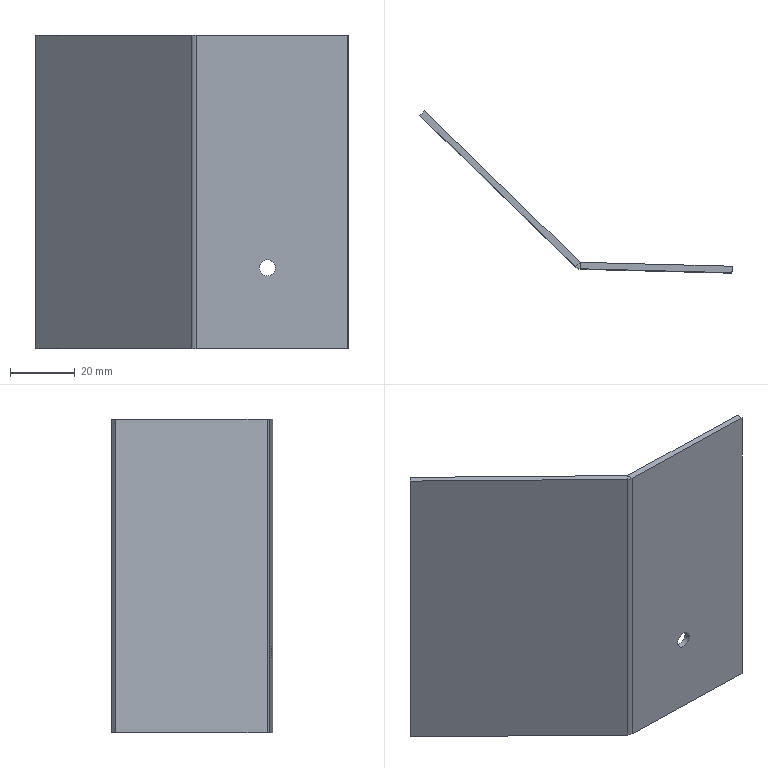Part | STEP file | Assembly TS-001-03 | 1 solid | 16 faces | box 96.717 x 50.15 x 97 mm | volume 22295 mm3 | plane 12 | cylinder 4 | commonest cylinder face diameters 5 x2 0.4 x1 4.4 x1
STEP:
#1=CARTESIAN_POINT('',(0.,0.,0.));
#2=DIRECTION('',(0.,0.,1.));
#3=DIRECTION('',(1.,0.,0.));
#4=AXIS2_PLACEMENT_3D('',#1,#2,#3);
#5=CARTESIAN_POINT('',(207.046,163.915,25.));
#6=VERTEX_POINT('',#5);
#7=CARTESIAN_POINT('',(207.098,165.914,25.));
#8=VERTEX_POINT('',#7);
#9=CARTESIAN_POINT('',(206.84,155.918,25.));
#10=DIRECTION('',(0.02576,0.9997,0.));
#11=VECTOR('',#10,1.);
#12=LINE('',#9,#11);
#13=CARTESIAN_POINT('',(209.34,155.853,25.));
#14=DIRECTION('',(0.02576,0.9997,0.));
#15=DIRECTION('',(-0.9997,0.02576,0.));
#16=AXIS2_PLACEMENT_3D('',#13,#14,#15);
#17=CYLINDRICAL_SURFACE('',#16,2.5);
#18=CARTESIAN_POINT('',(6.283,0.));
#19=DIRECTION('',(0.,1.));
#20=VECTOR('',#19,1.);
#21=LINE('',#18,#20);
#22=(GEOMETRIC_REPRESENTATION_CONTEXT(2)PARAMETRIC_REPRESENTATION_CONTEXT()REPRESENTATION_CONTEXT('',''));
#23=DEFINITIONAL_REPRESENTATION('',(#21),#22);
#24=PCURVE('',#17,#23);
#25=CARTESIAN_POINT('',(209.34,155.853,25.));
#26=DIRECTION('',(0.02576,0.9997,0.));
#27=DIRECTION('',(-0.9997,0.02576,0.));
#28=AXIS2_PLACEMENT_3D('',#25,#26,#27);
#29=CYLINDRICAL_SURFACE('',#28,2.5);
#30=CARTESIAN_POINT('',(0.,0.));
#31=DIRECTION('',(0.,1.));
#32=VECTOR('',#31,1.);
#33=LINE('',#30,#32);
#34=(GEOMETRIC_REPRESENTATION_CONTEXT(2)PARAMETRIC_REPRESENTATION_CONTEXT()REPRESENTATION_CONTEXT('',''));
#35=DEFINITIONAL_REPRESENTATION('',(#33),#34);
#36=PCURVE('',#29,#35);
#37=SURFACE_CURVE('',#12,(#24,#36),.PCURVE_S1.);
#38=EDGE_CURVE('',#6,#8,#37,.T.);
#39=ORIENTED_EDGE('',*,*,#38,.T.);
#40=CARTESIAN_POINT('',(212.096,165.785,25.));
#41=VERTEX_POINT('',#40);
#42=CARTESIAN_POINT('',(209.597,165.85,25.));
#43=DIRECTION('',(0.02576,0.9997,0.));
#44=DIRECTION('',(-0.9997,0.02576,0.));
#45=AXIS2_PLACEMENT_3D('',#42,#43,#44);
#46=CIRCLE('',#45,2.5);
#47=CARTESIAN_POINT('',(0.,10.));
#48=DIRECTION('',(1.,0.));
#49=VECTOR('',#48,1.);
#50=LINE('',#47,#49);
#51=(GEOMETRIC_REPRESENTATION_CONTEXT(2)PARAMETRIC_REPRESENTATION_CONTEXT()REPRESENTATION_CONTEXT('',''));
#52=DEFINITIONAL_REPRESENTATION('',(#50),#51);
#53=PCURVE('',#17,#52);
#54=CARTESIAN_POINT('',(234.589,165.206,97.));
#55=DIRECTION('',(-0.02576,-0.9997,0.));
#56=DIRECTION('',(0.9997,-0.02576,0.));
#57=AXIS2_PLACEMENT_3D('',#54,#55,#56);
#58=PLANE('',#57);
#59=CARTESIAN_POINT('',(-27.5,-72.));
#60=CARTESIAN_POINT('',(-27.5,-67.67));
#61=CARTESIAN_POINT('',(-23.75,-69.835));
#62=CARTESIAN_POINT('',(-20.,-72.));
#63=CARTESIAN_POINT('',(-23.75,-74.165));
#64=CARTESIAN_POINT('',(-27.5,-76.33));
#65=CARTESIAN_POINT('',(-27.5,-72.));
#66=(BOUNDED_CURVE()B_SPLINE_CURVE(2,(#59,#60,#61,#62,#63,#64,#65),.UNSPECIFIED.,.T.,.F.)B_SPLINE_CURVE_WITH_KNOTS((1,2,2,2,2,1),(-2.094,0.,2.094,4.189,6.283,8.378),.UNSPECIFIED.)CURVE()GEOMETRIC_REPRESENTATION_ITEM()RATIONAL_B_SPLINE_CURVE((1.,0.5,1.,0.5,1.,0.5,1.))REPRESENTATION_ITEM(''));
#67=(GEOMETRIC_REPRESENTATION_CONTEXT(2)PARAMETRIC_REPRESENTATION_CONTEXT()REPRESENTATION_CONTEXT('',''));
#68=DEFINITIONAL_REPRESENTATION('',(#66),#67);
#69=PCURVE('',#58,#68);
#70=SURFACE_CURVE('',#46,(#53,#69),.PCURVE_S1.);
#71=EDGE_CURVE('',#41,#8,#70,.T.);
#72=ORIENTED_EDGE('',*,*,#71,.F.);
#73=CARTESIAN_POINT('',(212.045,163.786,25.));
#74=VERTEX_POINT('',#73);
#75=CARTESIAN_POINT('',(211.839,155.789,25.));
#76=DIRECTION('',(0.02576,0.9997,0.));
#77=VECTOR('',#76,1.);
#78=LINE('',#75,#77);
#79=CARTESIAN_POINT('',(3.142,0.));
#80=DIRECTION('',(0.,1.));
#81=VECTOR('',#80,1.);
#82=LINE('',#79,#81);
#83=(GEOMETRIC_REPRESENTATION_CONTEXT(2)PARAMETRIC_REPRESENTATION_CONTEXT()REPRESENTATION_CONTEXT('',''));
#84=DEFINITIONAL_REPRESENTATION('',(#82),#83);
#85=PCURVE('',#17,#84);
#86=CARTESIAN_POINT('',(3.142,0.));
#87=DIRECTION('',(0.,1.));
#88=VECTOR('',#87,1.);
#89=LINE('',#86,#88);
#90=(GEOMETRIC_REPRESENTATION_CONTEXT(2)PARAMETRIC_REPRESENTATION_CONTEXT()REPRESENTATION_CONTEXT('',''));
#91=DEFINITIONAL_REPRESENTATION('',(#89),#90);
#92=PCURVE('',#29,#91);
#93=SURFACE_CURVE('',#78,(#85,#92),.PCURVE_S1.);
#94=EDGE_CURVE('',#74,#41,#93,.T.);
#95=ORIENTED_EDGE('',*,*,#94,.F.);
#96=CARTESIAN_POINT('',(209.546,163.85,25.));
#97=DIRECTION('',(-0.02576,-0.9997,0.));
#98=DIRECTION('',(0.9997,-0.02576,0.));
#99=AXIS2_PLACEMENT_3D('',#96,#97,#98);
#100=CIRCLE('',#99,2.5);
#101=CARTESIAN_POINT('',(9.425,8.));
#102=DIRECTION('',(-1.,0.));
#103=VECTOR('',#102,1.);
#104=LINE('',#101,#103);
#105=(GEOMETRIC_REPRESENTATION_CONTEXT(2)PARAMETRIC_REPRESENTATION_CONTEXT()REPRESENTATION_CONTEXT('',''));
#106=DEFINITIONAL_REPRESENTATION('',(#104),#105);
#107=PCURVE('',#17,#106);
#108=CARTESIAN_POINT('',(234.537,163.207,97.));
#109=DIRECTION('',(-0.02576,-0.9997,0.));
#110=DIRECTION('',(0.9997,-0.02576,0.));
#111=AXIS2_PLACEMENT_3D('',#108,#109,#110);
#112=PLANE('',#111);
#113=CARTESIAN_POINT('',(-25.,-72.));
#114=DIRECTION('',(1.,0.));
#115=AXIS2_PLACEMENT_2D('',#113,#114);
#116=CIRCLE('',#115,2.5);
#117=(GEOMETRIC_REPRESENTATION_CONTEXT(2)PARAMETRIC_REPRESENTATION_CONTEXT()REPRESENTATION_CONTEXT('',''));
#118=DEFINITIONAL_REPRESENTATION('',(#116),#117);
#119=PCURVE('',#112,#118);
#120=SURFACE_CURVE('',#100,(#107,#119),.PCURVE_S1.);
#121=EDGE_CURVE('',#6,#74,#120,.T.);
#122=ORIENTED_EDGE('',*,*,#121,.F.);
#123=EDGE_LOOP('',(#39,#72,#95,#122));
#124=FACE_BOUND('',#123,.F.);
#125=ADVANCED_FACE('',(#124),#17,.F.);
#126=CARTESIAN_POINT('',(186.126,165.037,97.));
#127=VERTEX_POINT('',#126);
#128=CARTESIAN_POINT('',(187.519,166.472,97.));
#129=VERTEX_POINT('',#128);
#130=CARTESIAN_POINT('',(186.126,165.037,97.));
#131=DIRECTION('',(0.6969,0.7172,0.));
#132=VECTOR('',#131,1.);
#133=LINE('',#130,#132);
#134=CARTESIAN_POINT('',(186.126,165.037,97.));
#135=DIRECTION('',(0.,0.,1.));
#136=DIRECTION('',(1.,0.,0.));
#137=AXIS2_PLACEMENT_3D('',#134,#135,#136);
#138=PLANE('',#137);
#139=CARTESIAN_POINT('',(0.,0.));
#140=DIRECTION('',(0.6969,0.7172));
#141=VECTOR('',#140,1.);
#142=LINE('',#139,#141);
#143=(GEOMETRIC_REPRESENTATION_CONTEXT(2)PARAMETRIC_REPRESENTATION_CONTEXT()REPRESENTATION_CONTEXT('',''));
#144=DEFINITIONAL_REPRESENTATION('',(#142),#143);
#145=PCURVE('',#138,#144);
#146=CARTESIAN_POINT('',(187.653,166.415,97.));
#147=DIRECTION('',(0.,0.,1.));
#148=DIRECTION('',(1.,0.,0.));
#149=AXIS2_PLACEMENT_3D('',#146,#147,#148);
#150=PLANE('',#149);
#151=CARTESIAN_POINT('',(-1.528,-1.378));
#152=DIRECTION('',(0.6969,0.7172));
#153=VECTOR('',#152,1.);
#154=LINE('',#151,#153);
#155=(GEOMETRIC_REPRESENTATION_CONTEXT(2)PARAMETRIC_REPRESENTATION_CONTEXT()REPRESENTATION_CONTEXT('',''));
#156=DEFINITIONAL_REPRESENTATION('',(#154),#155);
#157=PCURVE('',#150,#156);
#158=SURFACE_CURVE('',#133,(#145,#157),.PCURVE_S1.);
#159=EDGE_CURVE('',#127,#129,#158,.T.);
#160=ORIENTED_EDGE('',*,*,#159,.F.);
#161=CARTESIAN_POINT('',(187.602,164.416,97.));
#162=VERTEX_POINT('',#161);
#163=CARTESIAN_POINT('',(187.659,166.615,97.));
#164=DIRECTION('',(0.,0.,-1.));
#165=DIRECTION('',(1.,0.,0.));
#166=AXIS2_PLACEMENT_3D('',#163,#164,#165);
#167=CIRCLE('',#166,2.2);
#168=CARTESIAN_POINT('',(3.733,1.578));
#169=CARTESIAN_POINT('',(3.733,-2.233));
#170=CARTESIAN_POINT('',(0.4331,-0.3274));
#171=CARTESIAN_POINT('',(-2.867,1.578));
#172=CARTESIAN_POINT('',(0.4331,3.483));
#173=CARTESIAN_POINT('',(3.733,5.388));
#174=CARTESIAN_POINT('',(3.733,1.578));
#175=(BOUNDED_CURVE()B_SPLINE_CURVE(2,(#168,#169,#170,#171,#172,#173,#174),.UNSPECIFIED.,.T.,.F.)B_SPLINE_CURVE_WITH_KNOTS((1,2,2,2,2,1),(-2.094,0.,2.094,4.189,6.283,8.378),.UNSPECIFIED.)CURVE()GEOMETRIC_REPRESENTATION_ITEM()RATIONAL_B_SPLINE_CURVE((1.,0.5,1.,0.5,1.,0.5,1.))REPRESENTATION_ITEM(''));
#176=(GEOMETRIC_REPRESENTATION_CONTEXT(2)PARAMETRIC_REPRESENTATION_CONTEXT()REPRESENTATION_CONTEXT('',''));
#177=DEFINITIONAL_REPRESENTATION('',(#175),#176);
#178=PCURVE('',#138,#177);
#179=CARTESIAN_POINT('',(187.659,166.615,97.));
#180=DIRECTION('',(0.,0.,-1.));
#181=DIRECTION('',(-1.,0.,0.));
#182=AXIS2_PLACEMENT_3D('',#179,#180,#181);
#183=CYLINDRICAL_SURFACE('',#182,2.2);
#184=CARTESIAN_POINT('',(3.142,0.));
#185=DIRECTION('',(1.,0.));
#186=VECTOR('',#185,1.);
#187=LINE('',#184,#186);
#188=(GEOMETRIC_REPRESENTATION_CONTEXT(2)PARAMETRIC_REPRESENTATION_CONTEXT()REPRESENTATION_CONTEXT('',''));
#189=DEFINITIONAL_REPRESENTATION('',(#187),#188);
#190=PCURVE('',#183,#189);
#191=SURFACE_CURVE('',#167,(#178,#190),.PCURVE_S1.);
#192=EDGE_CURVE('',#162,#127,#191,.T.);
#193=ORIENTED_EDGE('',*,*,#192,.F.);
#194=CARTESIAN_POINT('',(187.653,166.415,97.));
#195=VERTEX_POINT('',#194);
#196=CARTESIAN_POINT('',(187.653,166.415,97.));
#197=DIRECTION('',(-0.02576,-0.9997,0.));
#198=VECTOR('',#197,1.);
#199=LINE('',#196,#198);
#200=CARTESIAN_POINT('',(1.528,1.378));
#201=DIRECTION('',(-0.02576,-0.9997));
#202=VECTOR('',#201,1.);
#203=LINE('',#200,#202);
#204=(GEOMETRIC_REPRESENTATION_CONTEXT(2)PARAMETRIC_REPRESENTATION_CONTEXT()REPRESENTATION_CONTEXT('',''));
#205=DEFINITIONAL_REPRESENTATION('',(#203),#204);
#206=PCURVE('',#138,#205);
#207=CARTESIAN_POINT('',(187.659,166.615,97.));
#208=DIRECTION('',(0.,0.,1.));
#209=DIRECTION('',(1.,0.,0.));
#210=AXIS2_PLACEMENT_3D('',#207,#208,#209);
#211=PLANE('',#210);
#212=CARTESIAN_POINT('',(-0.005151,-0.1999));
#213=DIRECTION('',(-0.02576,-0.9997));
#214=VECTOR('',#213,1.);
#215=LINE('',#212,#214);
#216=(GEOMETRIC_REPRESENTATION_CONTEXT(2)PARAMETRIC_REPRESENTATION_CONTEXT()REPRESENTATION_CONTEXT('',''));
#217=DEFINITIONAL_REPRESENTATION('',(#215),#216);
#218=PCURVE('',#211,#217);
#219=SURFACE_CURVE('',#199,(#206,#218),.PCURVE_S1.);
#220=EDGE_CURVE('',#195,#162,#219,.T.);
#221=ORIENTED_EDGE('',*,*,#220,.F.);
#222=CARTESIAN_POINT('',(187.659,166.615,97.));
#223=DIRECTION('',(0.,0.,-1.));
#224=DIRECTION('',(1.,0.,0.));
#225=AXIS2_PLACEMENT_3D('',#222,#223,#224);
#226=CIRCLE('',#225,0.2);
#227=CARTESIAN_POINT('',(1.733,1.578));
#228=CARTESIAN_POINT('',(1.733,1.231));
#229=CARTESIAN_POINT('',(1.433,1.405));
#230=CARTESIAN_POINT('',(1.133,1.578));
#231=CARTESIAN_POINT('',(1.433,1.751));
#232=CARTESIAN_POINT('',(1.733,1.924));
#233=CARTESIAN_POINT('',(1.733,1.578));
#234=(BOUNDED_CURVE()B_SPLINE_CURVE(2,(#227,#228,#229,#230,#231,#232,#233),.UNSPECIFIED.,.T.,.F.)B_SPLINE_CURVE_WITH_KNOTS((1,2,2,2,2,1),(-2.094,0.,2.094,4.189,6.283,8.378),.UNSPECIFIED.)CURVE()GEOMETRIC_REPRESENTATION_ITEM()RATIONAL_B_SPLINE_CURVE((1.,0.5,1.,0.5,1.,0.5,1.))REPRESENTATION_ITEM(''));
#235=(GEOMETRIC_REPRESENTATION_CONTEXT(2)PARAMETRIC_REPRESENTATION_CONTEXT()REPRESENTATION_CONTEXT('',''));
#236=DEFINITIONAL_REPRESENTATION('',(#234),#235);
#237=PCURVE('',#138,#236);
#238=CARTESIAN_POINT('',(187.659,166.615,97.));
#239=DIRECTION('',(0.,0.,-1.));
#240=DIRECTION('',(-1.,0.,0.));
#241=AXIS2_PLACEMENT_3D('',#238,#239,#240);
#242=CYLINDRICAL_SURFACE('',#241,0.2);
#243=CARTESIAN_POINT('',(3.142,0.));
#244=DIRECTION('',(1.,0.));
#245=VECTOR('',#244,1.);
#246=LINE('',#243,#245);
#247=(GEOMETRIC_REPRESENTATION_CONTEXT(2)PARAMETRIC_REPRESENTATION_CONTEXT()REPRESENTATION_CONTEXT('',''));
#248=DEFINITIONAL_REPRESENTATION('',(#246),#247);
#249=PCURVE('',#242,#248);
#250=SURFACE_CURVE('',#226,(#237,#249),.PCURVE_S1.);
#251=EDGE_CURVE('',#195,#129,#250,.T.);
#252=ORIENTED_EDGE('',*,*,#251,.T.);
#253=EDGE_LOOP('',(#160,#193,#221,#252));
#254=FACE_BOUND('',#253,.T.);
#255=ADVANCED_FACE('',(#254),#138,.T.);
#256=CARTESIAN_POINT('',(137.872,211.922,97.));
#257=VERTEX_POINT('',#256);
#258=CARTESIAN_POINT('',(186.742,164.438,97.));
#259=DIRECTION('',(-0.7172,0.6969,0.));
#260=VECTOR('',#259,1.);
#261=LINE('',#258,#260);
#262=CARTESIAN_POINT('',(-0.9112,-1.977));
#263=DIRECTION('',(-0.7172,0.6969));
#264=VECTOR('',#263,1.);
#265=LINE('',#262,#264);
#266=(GEOMETRIC_REPRESENTATION_CONTEXT(2)PARAMETRIC_REPRESENTATION_CONTEXT()REPRESENTATION_CONTEXT('',''));
#267=DEFINITIONAL_REPRESENTATION('',(#265),#266);
#268=PCURVE('',#150,#267);
#269=CARTESIAN_POINT('',(186.742,164.438,97.));
#270=DIRECTION('',(-0.6969,-0.7172,0.));
#271=DIRECTION('',(0.7172,-0.6969,0.));
#272=AXIS2_PLACEMENT_3D('',#269,#270,#271);
#273=PLANE('',#272);
#274=CARTESIAN_POINT('',(0.,0.));
#275=DIRECTION('',(-1.,0.));
#276=VECTOR('',#275,1.);
#277=LINE('',#274,#276);
#278=(GEOMETRIC_REPRESENTATION_CONTEXT(2)PARAMETRIC_REPRESENTATION_CONTEXT()REPRESENTATION_CONTEXT('',''));
#279=DEFINITIONAL_REPRESENTATION('',(#277),#278);
#280=PCURVE('',#273,#279);
#281=SURFACE_CURVE('',#261,(#268,#280),.PCURVE_S1.);
#282=EDGE_CURVE('',#127,#257,#281,.T.);
#283=ORIENTED_EDGE('',*,*,#282,.F.);
#284=ORIENTED_EDGE('',*,*,#159,.T.);
#285=CARTESIAN_POINT('',(139.266,213.357,97.));
#286=VERTEX_POINT('',#285);
#287=CARTESIAN_POINT('',(188.136,165.872,97.));
#288=DIRECTION('',(-0.7172,0.6969,0.));
#289=VECTOR('',#288,1.);
#290=LINE('',#287,#289);
#291=CARTESIAN_POINT('',(0.4825,-0.5428));
#292=DIRECTION('',(-0.7172,0.6969));
#293=VECTOR('',#292,1.);
#294=LINE('',#291,#293);
#295=(GEOMETRIC_REPRESENTATION_CONTEXT(2)PARAMETRIC_REPRESENTATION_CONTEXT()REPRESENTATION_CONTEXT('',''));
#296=DEFINITIONAL_REPRESENTATION('',(#294),#295);
#297=PCURVE('',#150,#296);
#298=CARTESIAN_POINT('',(188.136,165.872,97.));
#299=DIRECTION('',(-0.6969,-0.7172,0.));
#300=DIRECTION('',(0.7172,-0.6969,0.));
#301=AXIS2_PLACEMENT_3D('',#298,#299,#300);
#302=PLANE('',#301);
#303=CARTESIAN_POINT('',(0.,0.));
#304=DIRECTION('',(-1.,0.));
#305=VECTOR('',#304,1.);
#306=LINE('',#303,#305);
#307=(GEOMETRIC_REPRESENTATION_CONTEXT(2)PARAMETRIC_REPRESENTATION_CONTEXT()REPRESENTATION_CONTEXT('',''));
#308=DEFINITIONAL_REPRESENTATION('',(#306),#307);
#309=PCURVE('',#302,#308);
#310=SURFACE_CURVE('',#290,(#297,#309),.PCURVE_S1.);
#311=EDGE_CURVE('',#129,#286,#310,.T.);
#312=ORIENTED_EDGE('',*,*,#311,.T.);
#313=CARTESIAN_POINT('',(137.872,211.922,97.));
#314=DIRECTION('',(0.6969,0.7172,0.));
#315=VECTOR('',#314,1.);
#316=LINE('',#313,#315);
#317=CARTESIAN_POINT('',(-49.781,45.507));
#318=DIRECTION('',(0.6969,0.7172));
#319=VECTOR('',#318,1.);
#320=LINE('',#317,#319);
#321=(GEOMETRIC_REPRESENTATION_CONTEXT(2)PARAMETRIC_REPRESENTATION_CONTEXT()REPRESENTATION_CONTEXT('',''));
#322=DEFINITIONAL_REPRESENTATION('',(#320),#321);
#323=PCURVE('',#150,#322);
#324=CARTESIAN_POINT('',(137.872,211.922,97.));
#325=DIRECTION('',(-0.7172,0.6969,0.));
#326=DIRECTION('',(-0.6969,-0.7172,0.));
#327=AXIS2_PLACEMENT_3D('',#324,#325,#326);
#328=PLANE('',#327);
#329=CARTESIAN_POINT('',(0.,0.));
#330=DIRECTION('',(-1.,0.));
#331=VECTOR('',#330,1.);
#332=LINE('',#329,#331);
#333=(GEOMETRIC_REPRESENTATION_CONTEXT(2)PARAMETRIC_REPRESENTATION_CONTEXT()REPRESENTATION_CONTEXT('',''));
#334=DEFINITIONAL_REPRESENTATION('',(#332),#333);
#335=PCURVE('',#328,#334);
#336=SURFACE_CURVE('',#316,(#323,#335),.PCURVE_S1.);
#337=EDGE_CURVE('',#257,#286,#336,.T.);
#338=ORIENTED_EDGE('',*,*,#337,.F.);
#339=EDGE_LOOP('',(#283,#284,#312,#338));
#340=FACE_BOUND('',#339,.T.);
#341=ADVANCED_FACE('',(#340),#150,.T.);
#342=CARTESIAN_POINT('',(187.602,164.416,0.));
#343=VERTEX_POINT('',#342);
#344=CARTESIAN_POINT('',(187.653,166.415,0.));
#345=VERTEX_POINT('',#344);
#346=CARTESIAN_POINT('',(187.602,164.416,0.));
#347=DIRECTION('',(0.02576,0.9997,0.));
#348=VECTOR('',#347,1.);
#349=LINE('',#346,#348);
#350=CARTESIAN_POINT('',(187.602,164.416,0.));
#351=DIRECTION('',(0.,0.,-1.));
#352=DIRECTION('',(-1.,0.,0.));
#353=AXIS2_PLACEMENT_3D('',#350,#351,#352);
#354=PLANE('',#353);
#355=CARTESIAN_POINT('',(0.,0.));
#356=DIRECTION('',(-0.02576,0.9997));
#357=VECTOR('',#356,1.);
#358=LINE('',#355,#357);
#359=(GEOMETRIC_REPRESENTATION_CONTEXT(2)PARAMETRIC_REPRESENTATION_CONTEXT()REPRESENTATION_CONTEXT('',''));
#360=DEFINITIONAL_REPRESENTATION('',(#358),#359);
#361=PCURVE('',#354,#360);
#362=CARTESIAN_POINT('',(187.519,166.472,0.));
#363=DIRECTION('',(0.,0.,-1.));
#364=DIRECTION('',(-1.,0.,0.));
#365=AXIS2_PLACEMENT_3D('',#362,#363,#364);
#366=PLANE('',#365);
#367=CARTESIAN_POINT('',(-0.08271,-2.056));
#368=DIRECTION('',(-0.02576,0.9997));
#369=VECTOR('',#368,1.);
#370=LINE('',#367,#369);
#371=(GEOMETRIC_REPRESENTATION_CONTEXT(2)PARAMETRIC_REPRESENTATION_CONTEXT()REPRESENTATION_CONTEXT('',''));
#372=DEFINITIONAL_REPRESENTATION('',(#370),#371);
#373=PCURVE('',#366,#372);
#374=SURFACE_CURVE('',#349,(#361,#373),.PCURVE_S1.);
#375=EDGE_CURVE('',#343,#345,#374,.T.);
#376=ORIENTED_EDGE('',*,*,#375,.F.);
#377=CARTESIAN_POINT('',(186.126,165.037,0.));
#378=VERTEX_POINT('',#377);
#379=CARTESIAN_POINT('',(187.659,166.615,0.));
#380=DIRECTION('',(0.,0.,-1.));
#381=DIRECTION('',(1.,0.,0.));
#382=AXIS2_PLACEMENT_3D('',#379,#380,#381);
#383=CIRCLE('',#382,2.2);
#384=CARTESIAN_POINT('',(-0.05666,2.199));
#385=DIRECTION('',(-1.,0.));
#386=AXIS2_PLACEMENT_2D('',#384,#385);
#387=CIRCLE('',#386,2.2);
#388=(GEOMETRIC_REPRESENTATION_CONTEXT(2)PARAMETRIC_REPRESENTATION_CONTEXT()REPRESENTATION_CONTEXT('',''));
#389=DEFINITIONAL_REPRESENTATION('',(#387),#388);
#390=PCURVE('',#354,#389);
#391=CARTESIAN_POINT('',(3.142,97.));
#392=DIRECTION('',(1.,0.));
#393=VECTOR('',#392,1.);
#394=LINE('',#391,#393);
#395=(GEOMETRIC_REPRESENTATION_CONTEXT(2)PARAMETRIC_REPRESENTATION_CONTEXT()REPRESENTATION_CONTEXT('',''));
#396=DEFINITIONAL_REPRESENTATION('',(#394),#395);
#397=PCURVE('',#183,#396);
#398=SURFACE_CURVE('',#383,(#390,#397),.PCURVE_S1.);
#399=EDGE_CURVE('',#343,#378,#398,.T.);
#400=ORIENTED_EDGE('',*,*,#399,.T.);
#401=CARTESIAN_POINT('',(187.519,166.472,0.));
#402=VERTEX_POINT('',#401);
#403=CARTESIAN_POINT('',(187.519,166.472,0.));
#404=DIRECTION('',(-0.6969,-0.7172,0.));
#405=VECTOR('',#404,1.);
#406=LINE('',#403,#405);
#407=CARTESIAN_POINT('',(0.08271,2.056));
#408=DIRECTION('',(0.6969,-0.7172));
#409=VECTOR('',#408,1.);
#410=LINE('',#407,#409);
#411=(GEOMETRIC_REPRESENTATION_CONTEXT(2)PARAMETRIC_REPRESENTATION_CONTEXT()REPRESENTATION_CONTEXT('',''));
#412=DEFINITIONAL_REPRESENTATION('',(#410),#411);
#413=PCURVE('',#354,#412);
#414=CARTESIAN_POINT('',(187.659,166.615,0.));
#415=DIRECTION('',(0.,0.,1.));
#416=DIRECTION('',(1.,0.,0.));
#417=AXIS2_PLACEMENT_3D('',#414,#415,#416);
#418=PLANE('',#417);
#419=CARTESIAN_POINT('',(-0.1394,-0.1434));
#420=DIRECTION('',(-0.6969,-0.7172));
#421=VECTOR('',#420,1.);
#422=LINE('',#419,#421);
#423=(GEOMETRIC_REPRESENTATION_CONTEXT(2)PARAMETRIC_REPRESENTATION_CONTEXT()REPRESENTATION_CONTEXT('',''));
#424=DEFINITIONAL_REPRESENTATION('',(#422),#423);
#425=PCURVE('',#418,#424);
#426=SURFACE_CURVE('',#406,(#413,#425),.PCURVE_S1.);
#427=EDGE_CURVE('',#402,#378,#426,.T.);
#428=ORIENTED_EDGE('',*,*,#427,.F.);
#429=CARTESIAN_POINT('',(187.659,166.615,0.));
#430=DIRECTION('',(0.,0.,-1.));
#431=DIRECTION('',(1.,0.,0.));
#432=AXIS2_PLACEMENT_3D('',#429,#430,#431);
#433=CIRCLE('',#432,0.2);
#434=CARTESIAN_POINT('',(-0.05666,2.199));
#435=DIRECTION('',(-1.,0.));
#436=AXIS2_PLACEMENT_2D('',#434,#435);
#437=CIRCLE('',#436,0.2);
#438=(GEOMETRIC_REPRESENTATION_CONTEXT(2)PARAMETRIC_REPRESENTATION_CONTEXT()REPRESENTATION_CONTEXT('',''));
#439=DEFINITIONAL_REPRESENTATION('',(#437),#438);
#440=PCURVE('',#354,#439);
#441=CARTESIAN_POINT('',(3.142,97.));
#442=DIRECTION('',(1.,0.));
#443=VECTOR('',#442,1.);
#444=LINE('',#441,#443);
#445=(GEOMETRIC_REPRESENTATION_CONTEXT(2)PARAMETRIC_REPRESENTATION_CONTEXT()REPRESENTATION_CONTEXT('',''));
#446=DEFINITIONAL_REPRESENTATION('',(#444),#445);
#447=PCURVE('',#242,#446);
#448=SURFACE_CURVE('',#433,(#440,#447),.PCURVE_S1.);
#449=EDGE_CURVE('',#345,#402,#448,.T.);
#450=ORIENTED_EDGE('',*,*,#449,.F.);
#451=EDGE_LOOP('',(#376,#400,#428,#450));
#452=FACE_BOUND('',#451,.T.);
#453=ADVANCED_FACE('',(#452),#354,.T.);
#454=CARTESIAN_POINT('',(234.537,163.207,0.));
#455=VERTEX_POINT('',#454);
#456=CARTESIAN_POINT('',(234.537,163.207,0.));
#457=DIRECTION('',(-0.9997,0.02576,0.));
#458=VECTOR('',#457,1.);
#459=LINE('',#456,#458);
#460=CARTESIAN_POINT('',(-47.018,-3.265));
#461=DIRECTION('',(0.9997,0.02576));
#462=VECTOR('',#461,1.);
#463=LINE('',#460,#462);
#464=(GEOMETRIC_REPRESENTATION_CONTEXT(2)PARAMETRIC_REPRESENTATION_CONTEXT()REPRESENTATION_CONTEXT('',''));
#465=DEFINITIONAL_REPRESENTATION('',(#463),#464);
#466=PCURVE('',#366,#465);
#467=CARTESIAN_POINT('',(0.,-97.));
#468=DIRECTION('',(-1.,0.));
#469=VECTOR('',#468,1.);
#470=LINE('',#467,#469);
#471=(GEOMETRIC_REPRESENTATION_CONTEXT(2)PARAMETRIC_REPRESENTATION_CONTEXT()REPRESENTATION_CONTEXT('',''));
#472=DEFINITIONAL_REPRESENTATION('',(#470),#471);
#473=PCURVE('',#112,#472);
#474=SURFACE_CURVE('',#459,(#466,#473),.PCURVE_S1.);
#475=EDGE_CURVE('',#455,#343,#474,.T.);
#476=ORIENTED_EDGE('',*,*,#475,.T.);
#477=ORIENTED_EDGE('',*,*,#375,.T.);
#478=CARTESIAN_POINT('',(234.589,165.206,0.));
#479=VERTEX_POINT('',#478);
#480=CARTESIAN_POINT('',(234.589,165.206,0.));
#481=DIRECTION('',(-0.9997,0.02576,0.));
#482=VECTOR('',#481,1.);
#483=LINE('',#480,#482);
#484=CARTESIAN_POINT('',(-47.07,-1.266));
#485=DIRECTION('',(0.9997,0.02576));
#486=VECTOR('',#485,1.);
#487=LINE('',#484,#486);
#488=(GEOMETRIC_REPRESENTATION_CONTEXT(2)PARAMETRIC_REPRESENTATION_CONTEXT()REPRESENTATION_CONTEXT('',''));
#489=DEFINITIONAL_REPRESENTATION('',(#487),#488);
#490=PCURVE('',#366,#489);
#491=CARTESIAN_POINT('',(0.,-97.));
#492=DIRECTION('',(-1.,0.));
#493=VECTOR('',#492,1.);
#494=LINE('',#491,#493);
#495=(GEOMETRIC_REPRESENTATION_CONTEXT(2)PARAMETRIC_REPRESENTATION_CONTEXT()REPRESENTATION_CONTEXT('',''));
#496=DEFINITIONAL_REPRESENTATION('',(#494),#495);
#497=PCURVE('',#58,#496);
#498=SURFACE_CURVE('',#483,(#490,#497),.PCURVE_S1.);
#499=EDGE_CURVE('',#479,#345,#498,.T.);
#500=ORIENTED_EDGE('',*,*,#499,.F.);
#501=CARTESIAN_POINT('',(234.589,165.206,0.));
#502=DIRECTION('',(-0.02576,-0.9997,0.));
#503=VECTOR('',#502,1.);
#504=LINE('',#501,#503);
#505=CARTESIAN_POINT('',(-47.07,-1.266));
#506=DIRECTION('',(0.02576,-0.9997));
#507=VECTOR('',#506,1.);
#508=LINE('',#505,#507);
#509=(GEOMETRIC_REPRESENTATION_CONTEXT(2)PARAMETRIC_REPRESENTATION_CONTEXT()REPRESENTATION_CONTEXT('',''));
#510=DEFINITIONAL_REPRESENTATION('',(#508),#509);
#511=PCURVE('',#366,#510);
#512=CARTESIAN_POINT('',(234.589,165.206,97.));
#513=DIRECTION('',(0.9997,-0.02576,0.));
#514=DIRECTION('',(0.02576,0.9997,0.));
#515=AXIS2_PLACEMENT_3D('',#512,#513,#514);
#516=PLANE('',#515);
#517=CARTESIAN_POINT('',(0.,-97.));
#518=DIRECTION('',(-1.,0.));
#519=VECTOR('',#518,1.);
#520=LINE('',#517,#519);
#521=(GEOMETRIC_REPRESENTATION_CONTEXT(2)PARAMETRIC_REPRESENTATION_CONTEXT()REPRESENTATION_CONTEXT('',''));
#522=DEFINITIONAL_REPRESENTATION('',(#520),#521);
#523=PCURVE('',#516,#522);
#524=SURFACE_CURVE('',#504,(#511,#523),.PCURVE_S1.);
#525=EDGE_CURVE('',#479,#455,#524,.T.);
#526=ORIENTED_EDGE('',*,*,#525,.T.);
#527=EDGE_LOOP('',(#476,#477,#500,#526));
#528=FACE_BOUND('',#527,.T.);
#529=ADVANCED_FACE('',(#528),#366,.T.);
#530=CARTESIAN_POINT('',(139.266,213.357,0.));
#531=VERTEX_POINT('',#530);
#532=CARTESIAN_POINT('',(188.136,165.872,0.));
#533=DIRECTION('',(-0.7172,0.6969,0.));
#534=VECTOR('',#533,1.);
#535=LINE('',#532,#534);
#536=CARTESIAN_POINT('',(0.,-97.));
#537=DIRECTION('',(-1.,0.));
#538=VECTOR('',#537,1.);
#539=LINE('',#536,#538);
#540=(GEOMETRIC_REPRESENTATION_CONTEXT(2)PARAMETRIC_REPRESENTATION_CONTEXT()REPRESENTATION_CONTEXT('',''));
#541=DEFINITIONAL_REPRESENTATION('',(#539),#540);
#542=PCURVE('',#302,#541);
#543=CARTESIAN_POINT('',(0.4774,-0.7427));
#544=DIRECTION('',(-0.7172,0.6969));
#545=VECTOR('',#544,1.);
#546=LINE('',#543,#545);
#547=(GEOMETRIC_REPRESENTATION_CONTEXT(2)PARAMETRIC_REPRESENTATION_CONTEXT()REPRESENTATION_CONTEXT('',''));
#548=DEFINITIONAL_REPRESENTATION('',(#546),#547);
#549=PCURVE('',#418,#548);
#550=SURFACE_CURVE('',#535,(#542,#549),.PCURVE_S1.);
#551=EDGE_CURVE('',#402,#531,#550,.T.);
#552=ORIENTED_EDGE('',*,*,#551,.T.);
#553=CARTESIAN_POINT('',(139.266,213.357,97.));
#554=DIRECTION('',(0.,0.,-1.));
#555=VECTOR('',#554,1.);
#556=LINE('',#553,#555);
#557=CARTESIAN_POINT('',(-68.14,0.));
#558=DIRECTION('',(0.,-1.));
#559=VECTOR('',#558,1.);
#560=LINE('',#557,#559);
#561=(GEOMETRIC_REPRESENTATION_CONTEXT(2)PARAMETRIC_REPRESENTATION_CONTEXT()REPRESENTATION_CONTEXT('',''));
#562=DEFINITIONAL_REPRESENTATION('',(#560),#561);
#563=PCURVE('',#302,#562);
#564=CARTESIAN_POINT('',(-2.,0.));
#565=DIRECTION('',(0.,-1.));
#566=VECTOR('',#565,1.);
#567=LINE('',#564,#566);
#568=(GEOMETRIC_REPRESENTATION_CONTEXT(2)PARAMETRIC_REPRESENTATION_CONTEXT()REPRESENTATION_CONTEXT('',''));
#569=DEFINITIONAL_REPRESENTATION('',(#567),#568);
#570=PCURVE('',#328,#569);
#571=SURFACE_CURVE('',#556,(#563,#570),.PCURVE_S1.);
#572=EDGE_CURVE('',#286,#531,#571,.T.);
#573=ORIENTED_EDGE('',*,*,#572,.F.);
#574=ORIENTED_EDGE('',*,*,#311,.F.);
#575=CARTESIAN_POINT('',(187.519,166.472,97.));
#576=DIRECTION('',(0.,0.,-1.));
#577=VECTOR('',#576,1.);
#578=LINE('',#575,#577);
#579=CARTESIAN_POINT('',(-0.86,0.));
#580=DIRECTION('',(0.,-1.));
#581=VECTOR('',#580,1.);
#582=LINE('',#579,#581);
#583=(GEOMETRIC_REPRESENTATION_CONTEXT(2)PARAMETRIC_REPRESENTATION_CONTEXT()REPRESENTATION_CONTEXT('',''));
#584=DEFINITIONAL_REPRESENTATION('',(#582),#583);
#585=PCURVE('',#302,#584);
#586=CARTESIAN_POINT('',(5.483,0.));
#587=DIRECTION('',(0.,1.));
#588=VECTOR('',#587,1.);
#589=LINE('',#586,#588);
#590=(GEOMETRIC_REPRESENTATION_CONTEXT(2)PARAMETRIC_REPRESENTATION_CONTEXT()REPRESENTATION_CONTEXT('',''));
#591=DEFINITIONAL_REPRESENTATION('',(#589),#590);
#592=PCURVE('',#242,#591);
#593=SURFACE_CURVE('',#578,(#585,#592),.PCURVE_S1.);
#594=EDGE_CURVE('',#129,#402,#593,.T.);
#595=ORIENTED_EDGE('',*,*,#594,.T.);
#596=EDGE_LOOP('',(#552,#573,#574,#595));
#597=FACE_BOUND('',#596,.T.);
#598=ADVANCED_FACE('',(#597),#302,.F.);
#599=CARTESIAN_POINT('',(137.872,211.922,0.));
#600=VERTEX_POINT('',#599);
#601=CARTESIAN_POINT('',(137.872,211.922,0.));
#602=DIRECTION('',(0.6969,0.7172,0.));
#603=VECTOR('',#602,1.);
#604=LINE('',#601,#603);
#605=CARTESIAN_POINT('',(0.,-97.));
#606=DIRECTION('',(-1.,0.));
#607=VECTOR('',#606,1.);
#608=LINE('',#605,#607);
#609=(GEOMETRIC_REPRESENTATION_CONTEXT(2)PARAMETRIC_REPRESENTATION_CONTEXT()REPRESENTATION_CONTEXT('',''));
#610=DEFINITIONAL_REPRESENTATION('',(#608),#609);
#611=PCURVE('',#328,#610);
#612=CARTESIAN_POINT('',(-49.787,45.307));
#613=DIRECTION('',(0.6969,0.7172));
#614=VECTOR('',#613,1.);
#615=LINE('',#612,#614);
#616=(GEOMETRIC_REPRESENTATION_CONTEXT(2)PARAMETRIC_REPRESENTATION_CONTEXT()REPRESENTATION_CONTEXT('',''));
#617=DEFINITIONAL_REPRESENTATION('',(#615),#616);
#618=PCURVE('',#418,#617);
#619=SURFACE_CURVE('',#604,(#611,#618),.PCURVE_S1.);
#620=EDGE_CURVE('',#600,#531,#619,.T.);
#621=ORIENTED_EDGE('',*,*,#620,.F.);
#622=CARTESIAN_POINT('',(137.872,211.922,97.));
#623=DIRECTION('',(0.,0.,-1.));
#624=VECTOR('',#623,1.);
#625=LINE('',#622,#624);
#626=CARTESIAN_POINT('',(0.,0.));
#627=DIRECTION('',(0.,-1.));
#628=VECTOR('',#627,1.);
#629=LINE('',#626,#628);
#630=(GEOMETRIC_REPRESENTATION_CONTEXT(2)PARAMETRIC_REPRESENTATION_CONTEXT()REPRESENTATION_CONTEXT('',''));
#631=DEFINITIONAL_REPRESENTATION('',(#629),#630);
#632=PCURVE('',#328,#631);
#633=CARTESIAN_POINT('',(-68.14,0.));
#634=DIRECTION('',(0.,-1.));
#635=VECTOR('',#634,1.);
#636=LINE('',#633,#635);
#637=(GEOMETRIC_REPRESENTATION_CONTEXT(2)PARAMETRIC_REPRESENTATION_CONTEXT()REPRESENTATION_CONTEXT('',''));
#638=DEFINITIONAL_REPRESENTATION('',(#636),#637);
#639=PCURVE('',#273,#638);
#640=SURFACE_CURVE('',#625,(#632,#639),.PCURVE_S1.);
#641=EDGE_CURVE('',#257,#600,#640,.T.);
#642=ORIENTED_EDGE('',*,*,#641,.F.);
#643=ORIENTED_EDGE('',*,*,#337,.T.);
#644=ORIENTED_EDGE('',*,*,#572,.T.);
#645=EDGE_LOOP('',(#621,#642,#643,#644));
#646=FACE_BOUND('',#645,.T.);
#647=ADVANCED_FACE('',(#646),#328,.T.);
#648=CARTESIAN_POINT('',(186.742,164.438,0.));
#649=DIRECTION('',(-0.7172,0.6969,0.));
#650=VECTOR('',#649,1.);
#651=LINE('',#648,#650);
#652=CARTESIAN_POINT('',(0.,-97.));
#653=DIRECTION('',(-1.,0.));
#654=VECTOR('',#653,1.);
#655=LINE('',#652,#654);
#656=(GEOMETRIC_REPRESENTATION_CONTEXT(2)PARAMETRIC_REPRESENTATION_CONTEXT()REPRESENTATION_CONTEXT('',''));
#657=DEFINITIONAL_REPRESENTATION('',(#655),#656);
#658=PCURVE('',#273,#657);
#659=CARTESIAN_POINT('',(-0.9163,-2.177));
#660=DIRECTION('',(-0.7172,0.6969));
#661=VECTOR('',#660,1.);
#662=LINE('',#659,#661);
#663=(GEOMETRIC_REPRESENTATION_CONTEXT(2)PARAMETRIC_REPRESENTATION_CONTEXT()REPRESENTATION_CONTEXT('',''));
#664=DEFINITIONAL_REPRESENTATION('',(#662),#663);
#665=PCURVE('',#418,#664);
#666=SURFACE_CURVE('',#651,(#658,#665),.PCURVE_S1.);
#667=EDGE_CURVE('',#378,#600,#666,.T.);
#668=ORIENTED_EDGE('',*,*,#667,.F.);
#669=CARTESIAN_POINT('',(186.126,165.037,97.));
#670=DIRECTION('',(0.,0.,-1.));
#671=VECTOR('',#670,1.);
#672=LINE('',#669,#671);
#673=CARTESIAN_POINT('',(-0.86,0.));
#674=DIRECTION('',(0.,-1.));
#675=VECTOR('',#674,1.);
#676=LINE('',#673,#675);
#677=(GEOMETRIC_REPRESENTATION_CONTEXT(2)PARAMETRIC_REPRESENTATION_CONTEXT()REPRESENTATION_CONTEXT('',''));
#678=DEFINITIONAL_REPRESENTATION('',(#676),#677);
#679=PCURVE('',#273,#678);
#680=CARTESIAN_POINT('',(5.483,0.));
#681=DIRECTION('',(0.,1.));
#682=VECTOR('',#681,1.);
#683=LINE('',#680,#682);
#684=(GEOMETRIC_REPRESENTATION_CONTEXT(2)PARAMETRIC_REPRESENTATION_CONTEXT()REPRESENTATION_CONTEXT('',''));
#685=DEFINITIONAL_REPRESENTATION('',(#683),#684);
#686=PCURVE('',#183,#685);
#687=SURFACE_CURVE('',#672,(#679,#686),.PCURVE_S1.);
#688=EDGE_CURVE('',#127,#378,#687,.T.);
#689=ORIENTED_EDGE('',*,*,#688,.F.);
#690=ORIENTED_EDGE('',*,*,#282,.T.);
#691=ORIENTED_EDGE('',*,*,#641,.T.);
#692=EDGE_LOOP('',(#668,#689,#690,#691));
#693=FACE_BOUND('',#692,.T.);
#694=ADVANCED_FACE('',(#693),#273,.T.);
#695=ORIENTED_EDGE('',*,*,#399,.F.);
#696=CARTESIAN_POINT('',(187.602,164.416,97.));
#697=DIRECTION('',(0.,0.,-1.));
#698=VECTOR('',#697,1.);
#699=LINE('',#696,#698);
#700=CARTESIAN_POINT('',(4.738,0.));
#701=DIRECTION('',(0.,1.));
#702=VECTOR('',#701,1.);
#703=LINE('',#700,#702);
#704=(GEOMETRIC_REPRESENTATION_CONTEXT(2)PARAMETRIC_REPRESENTATION_CONTEXT()REPRESENTATION_CONTEXT('',''));
#705=DEFINITIONAL_REPRESENTATION('',(#703),#704);
#706=PCURVE('',#183,#705);
#707=CARTESIAN_POINT('',(-46.951,0.));
#708=DIRECTION('',(0.,-1.));
#709=VECTOR('',#708,1.);
#710=LINE('',#707,#709);
#711=(GEOMETRIC_REPRESENTATION_CONTEXT(2)PARAMETRIC_REPRESENTATION_CONTEXT()REPRESENTATION_CONTEXT('',''));
#712=DEFINITIONAL_REPRESENTATION('',(#710),#711);
#713=PCURVE('',#112,#712);
#714=SURFACE_CURVE('',#699,(#706,#713),.PCURVE_S1.);
#715=EDGE_CURVE('',#162,#343,#714,.T.);
#716=ORIENTED_EDGE('',*,*,#715,.F.);
#717=ORIENTED_EDGE('',*,*,#192,.T.);
#718=ORIENTED_EDGE('',*,*,#688,.T.);
#719=EDGE_LOOP('',(#695,#716,#717,#718));
#720=FACE_BOUND('',#719,.T.);
#721=ADVANCED_FACE('',(#720),#183,.T.);
#722=ORIENTED_EDGE('',*,*,#121,.F.);
#723=CARTESIAN_POINT('',(209.546,163.85,25.));
#724=DIRECTION('',(-0.02576,-0.9997,0.));
#725=DIRECTION('',(0.9997,-0.02576,0.));
#726=AXIS2_PLACEMENT_3D('',#723,#724,#725);
#727=CIRCLE('',#726,2.5);
#728=CARTESIAN_POINT('',(-25.,-72.));
#729=DIRECTION('',(1.,0.));
#730=AXIS2_PLACEMENT_2D('',#728,#729);
#731=CIRCLE('',#730,2.5);
#732=(GEOMETRIC_REPRESENTATION_CONTEXT(2)PARAMETRIC_REPRESENTATION_CONTEXT()REPRESENTATION_CONTEXT('',''));
#733=DEFINITIONAL_REPRESENTATION('',(#731),#732);
#734=PCURVE('',#112,#733);
#735=CARTESIAN_POINT('',(3.142,8.));
#736=DIRECTION('',(-1.,0.));
#737=VECTOR('',#736,1.);
#738=LINE('',#735,#737);
#739=(GEOMETRIC_REPRESENTATION_CONTEXT(2)PARAMETRIC_REPRESENTATION_CONTEXT()REPRESENTATION_CONTEXT('',''));
#740=DEFINITIONAL_REPRESENTATION('',(#738),#739);
#741=PCURVE('',#29,#740);
#742=SURFACE_CURVE('',#727,(#734,#741),.PCURVE_S1.);
#743=EDGE_CURVE('',#74,#6,#742,.T.);
#744=ORIENTED_EDGE('',*,*,#743,.F.);
#745=EDGE_LOOP('',(#722,#744));
#746=FACE_BOUND('',#745,.T.);
#747=ORIENTED_EDGE('',*,*,#475,.F.);
#748=CARTESIAN_POINT('',(234.537,163.207,97.));
#749=VERTEX_POINT('',#748);
#750=CARTESIAN_POINT('',(234.537,163.207,97.));
#751=DIRECTION('',(0.,0.,-1.));
#752=VECTOR('',#751,1.);
#753=LINE('',#750,#752);
#754=CARTESIAN_POINT('',(0.,0.));
#755=DIRECTION('',(0.,-1.));
#756=VECTOR('',#755,1.);
#757=LINE('',#754,#756);
#758=(GEOMETRIC_REPRESENTATION_CONTEXT(2)PARAMETRIC_REPRESENTATION_CONTEXT()REPRESENTATION_CONTEXT('',''));
#759=DEFINITIONAL_REPRESENTATION('',(#757),#758);
#760=PCURVE('',#112,#759);
#761=CARTESIAN_POINT('',(-2.,0.));
#762=DIRECTION('',(0.,-1.));
#763=VECTOR('',#762,1.);
#764=LINE('',#761,#763);
#765=(GEOMETRIC_REPRESENTATION_CONTEXT(2)PARAMETRIC_REPRESENTATION_CONTEXT()REPRESENTATION_CONTEXT('',''));
#766=DEFINITIONAL_REPRESENTATION('',(#764),#765);
#767=PCURVE('',#516,#766);
#768=SURFACE_CURVE('',#753,(#760,#767),.PCURVE_S1.);
#769=EDGE_CURVE('',#749,#455,#768,.T.);
#770=ORIENTED_EDGE('',*,*,#769,.F.);
#771=CARTESIAN_POINT('',(234.537,163.207,97.));
#772=DIRECTION('',(-0.9997,0.02576,0.));
#773=VECTOR('',#772,1.);
#774=LINE('',#771,#773);
#775=CARTESIAN_POINT('',(0.,0.));
#776=DIRECTION('',(-1.,0.));
#777=VECTOR('',#776,1.);
#778=LINE('',#775,#777);
#779=(GEOMETRIC_REPRESENTATION_CONTEXT(2)PARAMETRIC_REPRESENTATION_CONTEXT()REPRESENTATION_CONTEXT('',''));
#780=DEFINITIONAL_REPRESENTATION('',(#778),#779);
#781=PCURVE('',#112,#780);
#782=CARTESIAN_POINT('',(46.879,-3.409));
#783=DIRECTION('',(-0.9997,0.02576));
#784=VECTOR('',#783,1.);
#785=LINE('',#782,#784);
#786=(GEOMETRIC_REPRESENTATION_CONTEXT(2)PARAMETRIC_REPRESENTATION_CONTEXT()REPRESENTATION_CONTEXT('',''));
#787=DEFINITIONAL_REPRESENTATION('',(#785),#786);
#788=PCURVE('',#211,#787);
#789=SURFACE_CURVE('',#774,(#781,#788),.PCURVE_S1.);
#790=EDGE_CURVE('',#749,#162,#789,.T.);
#791=ORIENTED_EDGE('',*,*,#790,.T.);
#792=ORIENTED_EDGE('',*,*,#715,.T.);
#793=EDGE_LOOP('',(#747,#770,#791,#792));
#794=FACE_BOUND('',#793,.T.);
#795=ADVANCED_FACE('',(#746,#794),#112,.T.);
#796=ORIENTED_EDGE('',*,*,#525,.F.);
#797=CARTESIAN_POINT('',(234.589,165.206,97.));
#798=VERTEX_POINT('',#797);
#799=CARTESIAN_POINT('',(234.589,165.206,97.));
#800=DIRECTION('',(0.,0.,-1.));
#801=VECTOR('',#800,1.);
#802=LINE('',#799,#801);
#803=CARTESIAN_POINT('',(0.,0.));
#804=DIRECTION('',(0.,-1.));
#805=VECTOR('',#804,1.);
#806=LINE('',#803,#805);
#807=(GEOMETRIC_REPRESENTATION_CONTEXT(2)PARAMETRIC_REPRESENTATION_CONTEXT()REPRESENTATION_CONTEXT('',''));
#808=DEFINITIONAL_REPRESENTATION('',(#806),#807);
#809=PCURVE('',#516,#808);
#810=CARTESIAN_POINT('',(0.,0.));
#811=DIRECTION('',(0.,-1.));
#812=VECTOR('',#811,1.);
#813=LINE('',#810,#812);
#814=(GEOMETRIC_REPRESENTATION_CONTEXT(2)PARAMETRIC_REPRESENTATION_CONTEXT()REPRESENTATION_CONTEXT('',''));
#815=DEFINITIONAL_REPRESENTATION('',(#813),#814);
#816=PCURVE('',#58,#815);
#817=SURFACE_CURVE('',#802,(#809,#816),.PCURVE_S1.);
#818=EDGE_CURVE('',#798,#479,#817,.T.);
#819=ORIENTED_EDGE('',*,*,#818,.F.);
#820=CARTESIAN_POINT('',(234.589,165.206,97.));
#821=DIRECTION('',(-0.02576,-0.9997,0.));
#822=VECTOR('',#821,1.);
#823=LINE('',#820,#822);
#824=CARTESIAN_POINT('',(0.,0.));
#825=DIRECTION('',(-1.,0.));
#826=VECTOR('',#825,1.);
#827=LINE('',#824,#826);
#828=(GEOMETRIC_REPRESENTATION_CONTEXT(2)PARAMETRIC_REPRESENTATION_CONTEXT()REPRESENTATION_CONTEXT('',''));
#829=DEFINITIONAL_REPRESENTATION('',(#827),#828);
#830=PCURVE('',#516,#829);
#831=CARTESIAN_POINT('',(46.93,-1.409));
#832=DIRECTION('',(-0.02576,-0.9997));
#833=VECTOR('',#832,1.);
#834=LINE('',#831,#833);
#835=(GEOMETRIC_REPRESENTATION_CONTEXT(2)PARAMETRIC_REPRESENTATION_CONTEXT()REPRESENTATION_CONTEXT('',''));
#836=DEFINITIONAL_REPRESENTATION('',(#834),#835);
#837=PCURVE('',#211,#836);
#838=SURFACE_CURVE('',#823,(#830,#837),.PCURVE_S1.);
#839=EDGE_CURVE('',#798,#749,#838,.T.);
#840=ORIENTED_EDGE('',*,*,#839,.T.);
#841=ORIENTED_EDGE('',*,*,#769,.T.);
#842=EDGE_LOOP('',(#796,#819,#840,#841));
#843=FACE_BOUND('',#842,.T.);
#844=ADVANCED_FACE('',(#843),#516,.T.);
#845=CARTESIAN_POINT('',(209.597,165.85,25.));
#846=DIRECTION('',(0.02576,0.9997,0.));
#847=DIRECTION('',(-0.9997,0.02576,0.));
#848=AXIS2_PLACEMENT_3D('',#845,#846,#847);
#849=CIRCLE('',#848,2.5);
#850=CARTESIAN_POINT('',(-27.5,-72.));
#851=CARTESIAN_POINT('',(-27.5,-67.67));
#852=CARTESIAN_POINT('',(-23.75,-69.835));
#853=CARTESIAN_POINT('',(-20.,-72.));
#854=CARTESIAN_POINT('',(-23.75,-74.165));
#855=CARTESIAN_POINT('',(-27.5,-76.33));
#856=CARTESIAN_POINT('',(-27.5,-72.));
#857=(BOUNDED_CURVE()B_SPLINE_CURVE(2,(#850,#851,#852,#853,#854,#855,#856),.UNSPECIFIED.,.T.,.F.)B_SPLINE_CURVE_WITH_KNOTS((1,2,2,2,2,1),(-2.094,0.,2.094,4.189,6.283,8.378),.UNSPECIFIED.)CURVE()GEOMETRIC_REPRESENTATION_ITEM()RATIONAL_B_SPLINE_CURVE((1.,0.5,1.,0.5,1.,0.5,1.))REPRESENTATION_ITEM(''));
#858=(GEOMETRIC_REPRESENTATION_CONTEXT(2)PARAMETRIC_REPRESENTATION_CONTEXT()REPRESENTATION_CONTEXT('',''));
#859=DEFINITIONAL_REPRESENTATION('',(#857),#858);
#860=PCURVE('',#58,#859);
#861=CARTESIAN_POINT('',(0.,10.));
#862=DIRECTION('',(1.,0.));
#863=VECTOR('',#862,1.);
#864=LINE('',#861,#863);
#865=(GEOMETRIC_REPRESENTATION_CONTEXT(2)PARAMETRIC_REPRESENTATION_CONTEXT()REPRESENTATION_CONTEXT('',''));
#866=DEFINITIONAL_REPRESENTATION('',(#864),#865);
#867=PCURVE('',#29,#866);
#868=SURFACE_CURVE('',#849,(#860,#867),.PCURVE_S1.);
#869=EDGE_CURVE('',#8,#41,#868,.T.);
#870=ORIENTED_EDGE('',*,*,#869,.F.);
#871=ORIENTED_EDGE('',*,*,#71,.F.);
#872=EDGE_LOOP('',(#870,#871));
#873=FACE_BOUND('',#872,.T.);
#874=ORIENTED_EDGE('',*,*,#499,.T.);
#875=CARTESIAN_POINT('',(187.653,166.415,97.));
#876=DIRECTION('',(0.,0.,-1.));
#877=VECTOR('',#876,1.);
#878=LINE('',#875,#877);
#879=CARTESIAN_POINT('',(-46.951,0.));
#880=DIRECTION('',(0.,-1.));
#881=VECTOR('',#880,1.);
#882=LINE('',#879,#881);
#883=(GEOMETRIC_REPRESENTATION_CONTEXT(2)PARAMETRIC_REPRESENTATION_CONTEXT()REPRESENTATION_CONTEXT('',''));
#884=DEFINITIONAL_REPRESENTATION('',(#882),#883);
#885=PCURVE('',#58,#884);
#886=CARTESIAN_POINT('',(4.738,0.));
#887=DIRECTION('',(0.,1.));
#888=VECTOR('',#887,1.);
#889=LINE('',#886,#888);
#890=(GEOMETRIC_REPRESENTATION_CONTEXT(2)PARAMETRIC_REPRESENTATION_CONTEXT()REPRESENTATION_CONTEXT('',''));
#891=DEFINITIONAL_REPRESENTATION('',(#889),#890);
#892=PCURVE('',#242,#891);
#893=SURFACE_CURVE('',#878,(#885,#892),.PCURVE_S1.);
#894=EDGE_CURVE('',#195,#345,#893,.T.);
#895=ORIENTED_EDGE('',*,*,#894,.F.);
#896=CARTESIAN_POINT('',(234.589,165.206,97.));
#897=DIRECTION('',(-0.9997,0.02576,0.));
#898=VECTOR('',#897,1.);
#899=LINE('',#896,#898);
#900=CARTESIAN_POINT('',(0.,0.));
#901=DIRECTION('',(-1.,0.));
#902=VECTOR('',#901,1.);
#903=LINE('',#900,#902);
#904=(GEOMETRIC_REPRESENTATION_CONTEXT(2)PARAMETRIC_REPRESENTATION_CONTEXT()REPRESENTATION_CONTEXT('',''));
#905=DEFINITIONAL_REPRESENTATION('',(#903),#904);
#906=PCURVE('',#58,#905);
#907=CARTESIAN_POINT('',(46.93,-1.409));
#908=DIRECTION('',(-0.9997,0.02576));
#909=VECTOR('',#908,1.);
#910=LINE('',#907,#909);
#911=(GEOMETRIC_REPRESENTATION_CONTEXT(2)PARAMETRIC_REPRESENTATION_CONTEXT()REPRESENTATION_CONTEXT('',''));
#912=DEFINITIONAL_REPRESENTATION('',(#910),#911);
#913=PCURVE('',#211,#912);
#914=SURFACE_CURVE('',#899,(#906,#913),.PCURVE_S1.);
#915=EDGE_CURVE('',#798,#195,#914,.T.);
#916=ORIENTED_EDGE('',*,*,#915,.F.);
#917=ORIENTED_EDGE('',*,*,#818,.T.);
#918=EDGE_LOOP('',(#874,#895,#916,#917));
#919=FACE_BOUND('',#918,.T.);
#920=ADVANCED_FACE('',(#873,#919),#58,.F.);
#921=ORIENTED_EDGE('',*,*,#894,.F.);
#922=ORIENTED_EDGE('',*,*,#251,.T.);
#923=ORIENTED_EDGE('',*,*,#594,.T.);
#924=ORIENTED_EDGE('',*,*,#449,.F.);
#925=EDGE_LOOP('',(#921,#922,#923,#924));
#926=FACE_BOUND('',#925,.F.);
#927=ADVANCED_FACE('',(#926),#242,.F.);
#928=ORIENTED_EDGE('',*,*,#915,.T.);
#929=ORIENTED_EDGE('',*,*,#220,.T.);
#930=ORIENTED_EDGE('',*,*,#790,.F.);
#931=ORIENTED_EDGE('',*,*,#839,.F.);
#932=EDGE_LOOP('',(#928,#929,#930,#931));
#933=FACE_BOUND('',#932,.T.);
#934=ADVANCED_FACE('',(#933),#211,.T.);
#935=ORIENTED_EDGE('',*,*,#551,.F.);
#936=ORIENTED_EDGE('',*,*,#427,.T.);
#937=ORIENTED_EDGE('',*,*,#667,.T.);
#938=ORIENTED_EDGE('',*,*,#620,.T.);
#939=EDGE_LOOP('',(#935,#936,#937,#938));
#940=FACE_BOUND('',#939,.T.);
#941=ADVANCED_FACE('',(#940),#418,.F.);
#942=ORIENTED_EDGE('',*,*,#869,.F.);
#943=ORIENTED_EDGE('',*,*,#38,.F.);
#944=ORIENTED_EDGE('',*,*,#743,.F.);
#945=ORIENTED_EDGE('',*,*,#94,.T.);
#946=EDGE_LOOP('',(#942,#943,#944,#945));
#947=FACE_BOUND('',#946,.F.);
#948=ADVANCED_FACE('',(#947),#29,.F.);
#949=CLOSED_SHELL('',(#125,#255,#341,#453,#529,#598,#647,#694,#721,#795,#844,#920,#927,#934,#941,#948));
#950=MANIFOLD_SOLID_BREP('',#949);
#951=(LENGTH_UNIT()NAMED_UNIT(*)SI_UNIT(.MILLI.,.METRE.));
#952=UNCERTAINTY_MEASURE_WITH_UNIT(LENGTH_MEASURE(0.0000001),#951,'','');
#953=(NAMED_UNIT(*)PLANE_ANGLE_UNIT()SI_UNIT($,.RADIAN.));
#954=(NAMED_UNIT(*)SI_UNIT($,.STERADIAN.)SOLID_ANGLE_UNIT());
#955=(GEOMETRIC_REPRESENTATION_CONTEXT(3)GLOBAL_UNCERTAINTY_ASSIGNED_CONTEXT((#952))GLOBAL_UNIT_ASSIGNED_CONTEXT((#951,#953,#954))REPRESENTATION_CONTEXT('',''));
#956=ADVANCED_BREP_SHAPE_REPRESENTATION('',(#4,#950),#955);